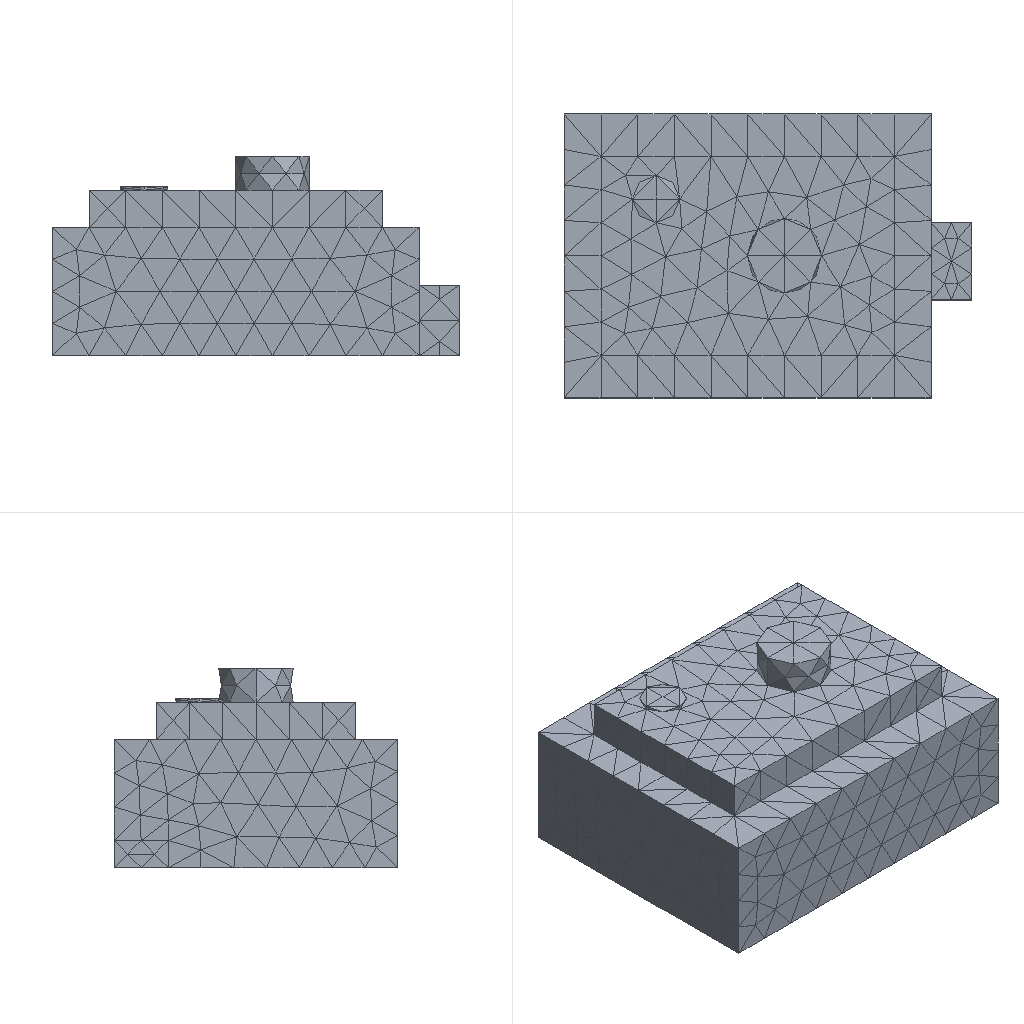Simulation study | ansys mapdl
Set-up summary:
category,name,step,type,value,unit,region
solver,ansys_mapdl
units,mm-N-s-tonne (MPa),,inferred,E=210000 density=
analysis,model,,static
mesh,nodes,,,5563
mesh,elements,,,3417
element_type,SOLID187,,,3417
material,mat 1,,E,210000
material,mat 1,,nu,0.3
load,,model,body load temp,,,all
load,,model,force,"1000 [dir=(0, 0, -1) n=400]",,node list
bc,,model,fixed,"[dofs=UX,UY,UZ n=6251]",,node list
Ansys APDL input file, long lists of numbers shortened:
/COM,ANSYS RELEASE 2026 R1           BUILD 26.1      UP20260202       09:09:04
/PREP7
/NOPR
/TITLE,2
ANTYPE, 0
*IF,_CDRDOFF,EQ,1,THEN     !if solid model was read in
_CDRDOFF=             !reset flag, numoffs already performed
*ELSE              !offset database for the following FE model
NUMOFF,NODE,     5563
NUMOFF,ELEM,     3417
NUMOFF,MAT ,        1
NUMOFF,TYPE,        1
*ENDIF
*SET,_RETURN ,  0.
*SET,_STATUS ,  0.
*SET,_UIQR   ,  400.
*SET,__FLOATPARAMETER__,  5563.
DOF,DELETE
ETBLOCK,        1,        1
(2i9,19a9)
        1      187        0        0        0        0        0        0        0        0        0        0        0        0        0        0        0        0        0        0        0
       -1
NBLOCK,6,SOLID,      5563,      5563
(3i9,6e21.13e3)
        1        0        0-3.8275000000000E+001 4.2000000000000E+001 8.0000000000000E+000
! (5562 more lines like these left out)
N,UNBL,LOC,       -1,
EBLOCK,19,SOLID,      3417,      3417
(19i10)
         1         1         1         1         0         0         0         0        10         0         1      1919       703      1920      1921      2272      2273      2274      2275
! (6833 more lines like these left out)
        -1
MPTEMP,UNBL, 1, 1,  0.    ,
MPDATA,UNBL, 1,EX  ,       1, 1,  210000.000    ,
MPTEMP,UNBL, 1, 1,  0.    ,
MPDATA,UNBL, 1,NUXY,       1, 1, 0.3    ,
MPTEMP,UNBL, 1, 1,  0.    ,
MPDATA,UNBL, 1,PRXY,       1, 1, 0.3    ,
EXTOPT,ATTR,      0,      0,      0
EXTOPT,ESIZE,  0,  0.
EXTOPT,ACLEAR,      0
TREF,  0.
IRLF,  0
BFUNIF,TEMP,_TINY
ACEL,  0.    ,  0.    ,  0.
OMEGA,  0.    ,  0.    ,  0.
DOMEGA,  0.    ,  0.    ,  0.
CGLOC,  0.    ,  0.    ,  0.
CGOMEGA,  0.    ,  0.    ,  0.
DCGOMG,  0.    ,  0.    ,  0.
KUSE,     0
TIME,  0.
ALPHAD,  0.
BETAD,  0.
DMPRAT,  0.
DMPSTR,  0.
CRPLIM, 0.1    ,   0
CRPLIM,  0.    ,   1
NCNV,     0, 1.000000000E+12,     0,  0.    ,  0.
NEQIT,     0
ERESX,DEFA
DBLOCK,      6251
(i9,a6,2(pg16.9))
        1  UX    0.00000000      0.00000000
! (6250 more lines like these left out)
       -1
FBLOCK,       400
(i9,a6,2(pg16.9))
      592  FZ   -2.50000000      0.00000000
! (399 more lines like these left out)
       -1
/GO
FINISH
Results summary:
result,analysis_type_db,,,static,unstated
result,n_sets,,,1,unstated
result,load_steps[0].set,load_step=1,,1,unstated
result,load_steps[0].substep,load_step=1,,1,unstated
result,load_steps[0].time,load_step=1,,1,unstated
result,load_steps[0].freq,load_step=1,,1,unstated
result,load_steps[0].max_usum,load_step=1,,0.0001168,unstated
result,load_steps[0].max_seqv,load_step=1,,8.316,unstated
result,load_steps[0].reaction_sum.FX,load_step=1,,-1.78551e-11,unstated
result,load_steps[0].reaction_sum.FY,load_step=1,,-3.10365e-11,unstated
result,load_steps[0].reaction_sum.FZ,load_step=1,,1000,unstated
result,load_steps[0].reaction_sum.MX,load_step=1,,0,unstated
result,load_steps[0].reaction_sum.MY,load_step=1,,0,unstated
result,load_steps[0].reaction_sum.MZ,load_step=1,,0,unstated
result,convergence,,,results present for all listed sets,unstated